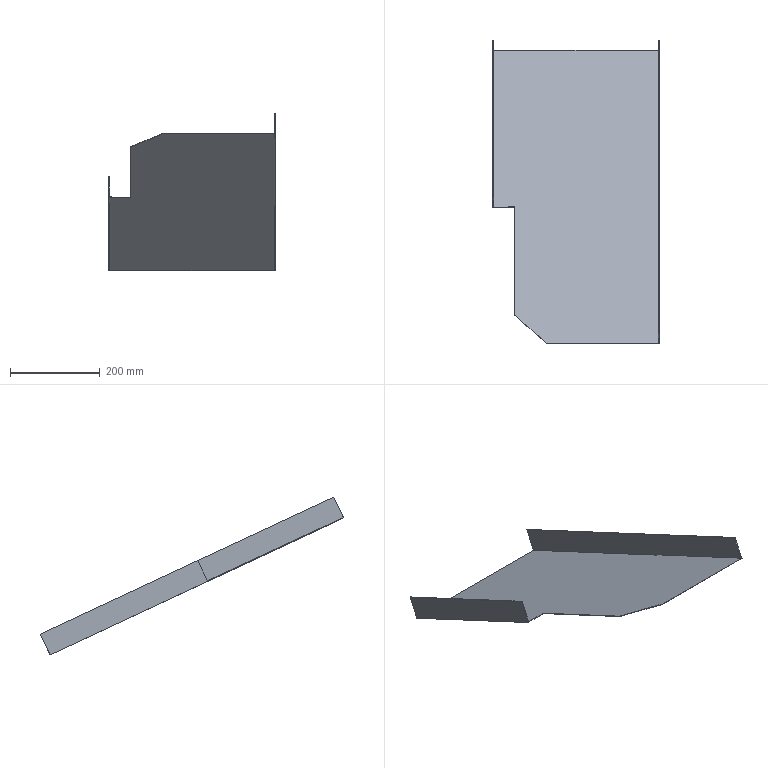Part | NX | features solid 2 | 1 solid | 14 faces | box 370 x 674.707 x 350.792 mm | volume 358626 mm3 | plane 13 | spline 1
STEP:
#1=CARTESIAN_POINT('',(542.,1102.315,-269.141));
#2=VERTEX_POINT('',#1);
#3=CARTESIAN_POINT('',(542.,751.83,-105.707));
#4=VERTEX_POINT('',#3);
#5=CARTESIAN_POINT('',(542.,630.423,-49.094));
#6=DIRECTION('',(0.,0.9063,-0.4226));
#7=VECTOR('',#6,1000.);
#8=LINE('',#5,#7);
#9=EDGE_CURVE('',#2,#4,#8,.F.);
#10=ORIENTED_EDGE('',*,*,#9,.T.);
#11=CARTESIAN_POINT('',(588.755,753.165,-106.33));
#12=VERTEX_POINT('',#11);
#13=CARTESIAN_POINT('',(588.755,753.165,-106.33));
#14=CARTESIAN_POINT('',(586.531,753.112,-106.305));
#15=CARTESIAN_POINT('',(582.277,753.007,-106.256));
#16=CARTESIAN_POINT('',(576.456,752.855,-106.185));
#17=CARTESIAN_POINT('',(572.547,752.747,-106.134));
#18=CARTESIAN_POINT('',(570.076,752.675,-106.101));
#19=CARTESIAN_POINT('',(568.579,752.63,-106.08));
#20=CARTESIAN_POINT('',(565.824,752.548,-106.042));
#21=CARTESIAN_POINT('',(562.091,752.434,-105.989));
#22=CARTESIAN_POINT('',(557.859,752.304,-105.928));
#23=CARTESIAN_POINT('',(554.361,752.195,-105.877));
#24=CARTESIAN_POINT('',(551.213,752.099,-105.832));
#25=CARTESIAN_POINT('',(547.008,751.973,-105.774));
#26=CARTESIAN_POINT('',(543.979,751.886,-105.733));
#27=CARTESIAN_POINT('',(542.,751.83,-105.707));
#28=B_SPLINE_CURVE_WITH_KNOTS('',3,(#13,#14,#15,#16,#17,#18,#19,#20,#21,#22,#23,#24,#25,#26,#27),.UNSPECIFIED.,.F.,.F.,(4,1,1,1,1,1,1,1,1,1,1,1,4),(0.,0.02122,0.04244,0.06367,0.06897,0.07428,0.08489,0.1061,0.1167,0.1273,0.1379,0.1486,0.1698),.UNSPECIFIED.);
#29=EDGE_CURVE('',#12,#4,#28,.T.);
#30=ORIENTED_EDGE('',*,*,#29,.F.);
#31=CARTESIAN_POINT('',(588.755,512.603,5.847));
#32=VERTEX_POINT('',#31);
#33=CARTESIAN_POINT('',(588.755,630.423,-49.094));
#34=DIRECTION('',(0.,-0.9063,0.4226));
#35=VECTOR('',#34,1000.);
#36=LINE('',#33,#35);
#37=EDGE_CURVE('',#32,#12,#36,.F.);
#38=ORIENTED_EDGE('',*,*,#37,.F.);
#39=CARTESIAN_POINT('',(658.755,449.161,35.43));
#40=VERTEX_POINT('',#39);
#41=CARTESIAN_POINT('',(-320.623,1336.778,-378.473));
#42=DIRECTION('',(0.7071,-0.6409,0.2988));
#43=VECTOR('',#42,1000.);
#44=LINE('',#41,#43);
#45=EDGE_CURVE('',#40,#32,#44,.F.);
#46=ORIENTED_EDGE('',*,*,#45,.F.);
#47=CARTESIAN_POINT('',(908.,449.161,35.43));
#48=VERTEX_POINT('',#47);
#49=CARTESIAN_POINT('',(-1100.,449.161,35.43));
#50=DIRECTION('',(1.,0.,0.));
#51=VECTOR('',#50,1000.);
#52=LINE('',#49,#51);
#53=EDGE_CURVE('',#48,#40,#52,.F.);
#54=ORIENTED_EDGE('',*,*,#53,.F.);
#55=CARTESIAN_POINT('',(908.,1102.315,-269.141));
#56=VERTEX_POINT('',#55);
#57=CARTESIAN_POINT('',(908.,630.423,-49.094));
#58=DIRECTION('',(0.,0.9063,-0.4226));
#59=VECTOR('',#58,1000.);
#60=LINE('',#57,#59);
#61=EDGE_CURVE('',#56,#48,#60,.F.);
#62=ORIENTED_EDGE('',*,*,#61,.F.);
#63=CARTESIAN_POINT('',(-1100.,1102.315,-269.141));
#64=DIRECTION('',(1.,0.,0.));
#65=VECTOR('',#64,1000.);
#66=LINE('',#63,#65);
#67=EDGE_CURVE('',#56,#2,#66,.F.);
#68=ORIENTED_EDGE('',*,*,#67,.T.);
#69=EDGE_LOOP('',(#10,#30,#38,#46,#54,#62,#68));
#70=FACE_BOUND('',#69,.T.);
#71=CARTESIAN_POINT('',(-1100.,630.423,-49.094));
#72=DIRECTION('',(0.,-0.4226,-0.9063));
#73=DIRECTION('',(0.,-0.9063,0.4226));
#74=AXIS2_PLACEMENT_3D('',#71,#72,#73);
#75=PLANE('',#74);
#76=ADVANCED_FACE('',(#70),#75,.F.);
#77=ORIENTED_EDGE('',*,*,#37,.T.);
#78=CARTESIAN_POINT('',(588.755,752.743,-107.236));
#79=VERTEX_POINT('',#78);
#80=CARTESIAN_POINT('',(588.755,753.165,-106.33));
#81=CARTESIAN_POINT('',(588.755,753.024,-106.632));
#82=CARTESIAN_POINT('',(588.755,752.883,-106.934));
#83=CARTESIAN_POINT('',(588.755,752.743,-107.236));
#84=B_SPLINE_CURVE_WITH_KNOTS('',3,(#80,#81,#82,#83),.UNSPECIFIED.,.F.,.F.,(4,4),(0.,1.),.UNSPECIFIED.);
#85=EDGE_CURVE('',#79,#12,#84,.F.);
#86=ORIENTED_EDGE('',*,*,#85,.F.);
#87=CARTESIAN_POINT('',(588.755,512.18,4.94));
#88=VERTEX_POINT('',#87);
#89=CARTESIAN_POINT('',(588.755,630.,-50.));
#90=DIRECTION('',(0.,-0.9063,0.4226));
#91=VECTOR('',#90,1000.);
#92=LINE('',#89,#91);
#93=EDGE_CURVE('',#88,#79,#92,.F.);
#94=ORIENTED_EDGE('',*,*,#93,.F.);
#95=CARTESIAN_POINT('',(588.755,512.18,4.94));
#96=DIRECTION('',(0.,-0.4226,-0.9063));
#97=VECTOR('',#96,1000.);
#98=LINE('',#95,#97);
#99=EDGE_CURVE('',#32,#88,#98,.T.);
#100=ORIENTED_EDGE('',*,*,#99,.F.);
#101=EDGE_LOOP('',(#77,#86,#94,#100));
#102=FACE_BOUND('',#101,.T.);
#103=CARTESIAN_POINT('',(588.755,630.,-50.));
#104=DIRECTION('',(-1.,0.,0.));
#105=DIRECTION('',(0.,0.,1.));
#106=AXIS2_PLACEMENT_3D('',#103,#104,#105);
#107=PLANE('',#106);
#108=ADVANCED_FACE('',(#102),#107,.T.);
#109=CARTESIAN_POINT('',(542.,751.407,-106.613));
#110=VERTEX_POINT('',#109);
#111=CARTESIAN_POINT('',(542.,751.407,-106.613));
#112=DIRECTION('',(0.,0.4226,0.9063));
#113=VECTOR('',#112,1000.);
#114=LINE('',#111,#113);
#115=EDGE_CURVE('',#4,#110,#114,.F.);
#116=ORIENTED_EDGE('',*,*,#115,.T.);
#117=CARTESIAN_POINT('',(588.755,752.743,-107.236));
#118=CARTESIAN_POINT('',(586.531,752.689,-107.211));
#119=CARTESIAN_POINT('',(582.277,752.584,-107.162));
#120=CARTESIAN_POINT('',(576.456,752.433,-107.091));
#121=CARTESIAN_POINT('',(572.547,752.324,-107.041));
#122=CARTESIAN_POINT('',(570.076,752.252,-107.007));
#123=CARTESIAN_POINT('',(568.579,752.208,-106.986));
#124=CARTESIAN_POINT('',(565.824,752.125,-106.948));
#125=CARTESIAN_POINT('',(562.091,752.012,-106.895));
#126=CARTESIAN_POINT('',(557.859,751.881,-106.834));
#127=CARTESIAN_POINT('',(554.361,751.773,-106.783));
#128=CARTESIAN_POINT('',(551.213,751.676,-106.739));
#129=CARTESIAN_POINT('',(547.008,751.55,-106.68));
#130=CARTESIAN_POINT('',(543.979,751.463,-106.639));
#131=CARTESIAN_POINT('',(542.,751.407,-106.613));
#132=B_SPLINE_CURVE_WITH_KNOTS('',3,(#117,#118,#119,#120,#121,#122,#123,#124,#125,#126,#127,#128,#129,#130,#131),.UNSPECIFIED.,.F.,.F.,(4,1,1,1,1,1,1,1,1,1,1,1,4),(0.,0.02122,0.04244,0.06367,0.06897,0.07428,0.08489,0.1061,0.1167,0.1273,0.1379,0.1486,0.1698),.UNSPECIFIED.);
#133=EDGE_CURVE('',#79,#110,#132,.T.);
#134=ORIENTED_EDGE('',*,*,#133,.F.);
#135=ORIENTED_EDGE('',*,*,#85,.T.);
#136=ORIENTED_EDGE('',*,*,#29,.T.);
#137=EDGE_LOOP('',(#116,#134,#135,#136));
#138=FACE_BOUND('',#137,.T.);
#139=CARTESIAN_POINT('',(588.755,752.743,-107.236));
#140=CARTESIAN_POINT('',(588.755,753.165,-106.33));
#141=CARTESIAN_POINT('',(586.531,752.689,-107.211));
#142=CARTESIAN_POINT('',(586.531,753.112,-106.305));
#143=CARTESIAN_POINT('',(582.277,752.584,-107.162));
#144=CARTESIAN_POINT('',(582.277,753.007,-106.256));
#145=CARTESIAN_POINT('',(576.456,752.433,-107.091));
#146=CARTESIAN_POINT('',(576.456,752.855,-106.185));
#147=CARTESIAN_POINT('',(572.547,752.324,-107.041));
#148=CARTESIAN_POINT('',(572.547,752.747,-106.134));
#149=CARTESIAN_POINT('',(570.076,752.252,-107.007));
#150=CARTESIAN_POINT('',(570.076,752.675,-106.101));
#151=CARTESIAN_POINT('',(568.579,752.208,-106.986));
#152=CARTESIAN_POINT('',(568.579,752.63,-106.08));
#153=CARTESIAN_POINT('',(565.824,752.125,-106.948));
#154=CARTESIAN_POINT('',(565.824,752.548,-106.042));
#155=CARTESIAN_POINT('',(562.091,752.012,-106.895));
#156=CARTESIAN_POINT('',(562.091,752.434,-105.989));
#157=CARTESIAN_POINT('',(557.859,751.881,-106.834));
#158=CARTESIAN_POINT('',(557.859,752.304,-105.928));
#159=CARTESIAN_POINT('',(554.361,751.773,-106.783));
#160=CARTESIAN_POINT('',(554.361,752.195,-105.877));
#161=CARTESIAN_POINT('',(551.213,751.676,-106.739));
#162=CARTESIAN_POINT('',(551.213,752.099,-105.832));
#163=CARTESIAN_POINT('',(547.008,751.55,-106.68));
#164=CARTESIAN_POINT('',(547.008,751.973,-105.774));
#165=CARTESIAN_POINT('',(543.979,751.463,-106.639));
#166=CARTESIAN_POINT('',(543.979,751.886,-105.733));
#167=CARTESIAN_POINT('',(542.,751.407,-106.613));
#168=CARTESIAN_POINT('',(542.,751.83,-105.707));
#169=B_SPLINE_SURFACE_WITH_KNOTS('',3,1,((#139,#140),(#141,#142),(#143,#144),(#145,#146),(#147,#148),(#149,#150),(#151,#152),(#153,#154),(#155,#156),(#157,#158),(#159,#160),(#161,#162),(#163,#164),(#165,#166),(#167,#168)),.SURF_OF_LINEAR_EXTRUSION.,.F.,.F.,.F.,(4,1,1,1,1,1,1,1,1,1,1,1,4),(2,2),(0.,0.02122,0.04244,0.06367,0.06897,0.07428,0.08489,0.1061,0.1167,0.1273,0.1379,0.1486,0.1698),(0.,1.),.UNSPECIFIED.);
#170=ADVANCED_FACE('',(#138),#169,.F.);
#171=ORIENTED_EDGE('',*,*,#67,.F.);
#172=CARTESIAN_POINT('',(908.,1123.446,-223.825));
#173=VERTEX_POINT('',#172);
#174=CARTESIAN_POINT('',(908.,1123.446,-223.825));
#175=DIRECTION('',(0.,-0.4226,-0.9063));
#176=VECTOR('',#175,1000.);
#177=LINE('',#174,#176);
#178=EDGE_CURVE('',#173,#56,#177,.T.);
#179=ORIENTED_EDGE('',*,*,#178,.F.);
#180=CARTESIAN_POINT('',(910.,1123.446,-223.825));
#181=VERTEX_POINT('',#180);
#182=CARTESIAN_POINT('',(910.,1123.446,-223.825));
#183=DIRECTION('',(1.,0.,0.));
#184=VECTOR('',#183,1000.);
#185=LINE('',#182,#184);
#186=EDGE_CURVE('',#181,#173,#185,.F.);
#187=ORIENTED_EDGE('',*,*,#186,.F.);
#188=CARTESIAN_POINT('',(910.,1101.892,-270.047));
#189=VERTEX_POINT('',#188);
#190=CARTESIAN_POINT('',(910.,1101.892,-270.047));
#191=DIRECTION('',(0.,0.4226,0.9063));
#192=VECTOR('',#191,1000.);
#193=LINE('',#190,#192);
#194=EDGE_CURVE('',#189,#181,#193,.T.);
#195=ORIENTED_EDGE('',*,*,#194,.F.);
#196=CARTESIAN_POINT('',(540.,1101.892,-270.047));
#197=VERTEX_POINT('',#196);
#198=CARTESIAN_POINT('',(-1100.,1101.892,-270.047));
#199=DIRECTION('',(1.,0.,0.));
#200=VECTOR('',#199,1000.);
#201=LINE('',#198,#200);
#202=EDGE_CURVE('',#189,#197,#201,.F.);
#203=ORIENTED_EDGE('',*,*,#202,.T.);
#204=CARTESIAN_POINT('',(540.,1123.446,-223.825));
#205=VERTEX_POINT('',#204);
#206=CARTESIAN_POINT('',(540.,1101.892,-270.047));
#207=DIRECTION('',(0.,-0.4226,-0.9063));
#208=VECTOR('',#207,1000.);
#209=LINE('',#206,#208);
#210=EDGE_CURVE('',#205,#197,#209,.T.);
#211=ORIENTED_EDGE('',*,*,#210,.F.);
#212=CARTESIAN_POINT('',(542.,1123.446,-223.825));
#213=VERTEX_POINT('',#212);
#214=CARTESIAN_POINT('',(540.,1123.446,-223.825));
#215=DIRECTION('',(1.,0.,0.));
#216=VECTOR('',#215,1000.);
#217=LINE('',#214,#216);
#218=EDGE_CURVE('',#213,#205,#217,.F.);
#219=ORIENTED_EDGE('',*,*,#218,.F.);
#220=CARTESIAN_POINT('',(542.,1101.892,-270.047));
#221=DIRECTION('',(0.,0.4226,0.9063));
#222=VECTOR('',#221,1000.);
#223=LINE('',#220,#222);
#224=EDGE_CURVE('',#2,#213,#223,.T.);
#225=ORIENTED_EDGE('',*,*,#224,.F.);
#226=EDGE_LOOP('',(#171,#179,#187,#195,#203,#211,#219,#225));
#227=FACE_BOUND('',#226,.T.);
#228=CARTESIAN_POINT('',(-1100.,1101.892,-270.047));
#229=DIRECTION('',(0.,-0.9063,0.4226));
#230=DIRECTION('',(0.,0.4226,0.9063));
#231=AXIS2_PLACEMENT_3D('',#228,#229,#230);
#232=PLANE('',#231);
#233=ADVANCED_FACE('',(#227),#232,.F.);
#234=CARTESIAN_POINT('',(910.,448.738,34.524));
#235=VERTEX_POINT('',#234);
#236=CARTESIAN_POINT('',(910.,470.292,80.745));
#237=VERTEX_POINT('',#236);
#238=CARTESIAN_POINT('',(910.,448.738,34.524));
#239=DIRECTION('',(0.,0.4226,0.9063));
#240=VECTOR('',#239,1000.);
#241=LINE('',#238,#240);
#242=EDGE_CURVE('',#235,#237,#241,.T.);
#243=ORIENTED_EDGE('',*,*,#242,.F.);
#244=CARTESIAN_POINT('',(910.,630.,-50.));
#245=DIRECTION('',(0.,-0.9063,0.4226));
#246=VECTOR('',#245,1000.);
#247=LINE('',#244,#246);
#248=EDGE_CURVE('',#235,#189,#247,.F.);
#249=ORIENTED_EDGE('',*,*,#248,.T.);
#250=ORIENTED_EDGE('',*,*,#194,.T.);
#251=CARTESIAN_POINT('',(910.,470.292,80.745));
#252=DIRECTION('',(0.,0.9063,-0.4226));
#253=VECTOR('',#252,1000.);
#254=LINE('',#251,#253);
#255=EDGE_CURVE('',#237,#181,#254,.T.);
#256=ORIENTED_EDGE('',*,*,#255,.F.);
#257=EDGE_LOOP('',(#243,#249,#250,#256));
#258=FACE_BOUND('',#257,.T.);
#259=CARTESIAN_POINT('',(910.,630.,-50.));
#260=DIRECTION('',(-1.,0.,0.));
#261=DIRECTION('',(0.,0.,1.));
#262=AXIS2_PLACEMENT_3D('',#259,#260,#261);
#263=PLANE('',#262);
#264=ADVANCED_FACE('',(#258),#263,.F.);
#265=ORIENTED_EDGE('',*,*,#242,.T.);
#266=CARTESIAN_POINT('',(908.,470.292,80.745));
#267=VERTEX_POINT('',#266);
#268=CARTESIAN_POINT('',(910.,470.292,80.745));
#269=DIRECTION('',(1.,0.,0.));
#270=VECTOR('',#269,1000.);
#271=LINE('',#268,#270);
#272=EDGE_CURVE('',#237,#267,#271,.F.);
#273=ORIENTED_EDGE('',*,*,#272,.T.);
#274=CARTESIAN_POINT('',(908.,470.292,80.745));
#275=DIRECTION('',(0.,-0.4226,-0.9063));
#276=VECTOR('',#275,1000.);
#277=LINE('',#274,#276);
#278=EDGE_CURVE('',#267,#48,#277,.T.);
#279=ORIENTED_EDGE('',*,*,#278,.T.);
#280=ORIENTED_EDGE('',*,*,#53,.T.);
#281=CARTESIAN_POINT('',(658.755,448.738,34.524));
#282=VERTEX_POINT('',#281);
#283=CARTESIAN_POINT('',(658.755,448.738,34.524));
#284=DIRECTION('',(0.,0.4226,0.9063));
#285=VECTOR('',#284,1000.);
#286=LINE('',#283,#285);
#287=EDGE_CURVE('',#282,#40,#286,.T.);
#288=ORIENTED_EDGE('',*,*,#287,.F.);
#289=CARTESIAN_POINT('',(-1100.,448.738,34.524));
#290=DIRECTION('',(-1.,0.,0.));
#291=VECTOR('',#290,1000.);
#292=LINE('',#289,#291);
#293=EDGE_CURVE('',#282,#235,#292,.F.);
#294=ORIENTED_EDGE('',*,*,#293,.T.);
#295=EDGE_LOOP('',(#265,#273,#279,#280,#288,#294));
#296=FACE_BOUND('',#295,.T.);
#297=CARTESIAN_POINT('',(-1100.,448.738,34.524));
#298=DIRECTION('',(0.,0.9063,-0.4226));
#299=DIRECTION('',(0.,-0.4226,-0.9063));
#300=AXIS2_PLACEMENT_3D('',#297,#298,#299);
#301=PLANE('',#300);
#302=ADVANCED_FACE('',(#296),#301,.F.);
#303=ORIENTED_EDGE('',*,*,#202,.F.);
#304=ORIENTED_EDGE('',*,*,#248,.F.);
#305=ORIENTED_EDGE('',*,*,#293,.F.);
#306=CARTESIAN_POINT('',(708.755,403.423,55.655));
#307=DIRECTION('',(-0.7071,0.6409,-0.2988));
#308=VECTOR('',#307,1000.);
#309=LINE('',#306,#308);
#310=EDGE_CURVE('',#88,#282,#309,.F.);
#311=ORIENTED_EDGE('',*,*,#310,.F.);
#312=ORIENTED_EDGE('',*,*,#93,.T.);
#313=ORIENTED_EDGE('',*,*,#133,.T.);
#314=CARTESIAN_POINT('',(542.,751.352,-106.587));
#315=VERTEX_POINT('',#314);
#316=CARTESIAN_POINT('',(542.,1101.892,-270.047));
#317=DIRECTION('',(0.,-0.9063,0.4226));
#318=VECTOR('',#317,1000.);
#319=LINE('',#316,#318);
#320=EDGE_CURVE('',#110,#315,#319,.T.);
#321=ORIENTED_EDGE('',*,*,#320,.T.);
#322=CARTESIAN_POINT('',(540.,751.352,-106.587));
#323=VERTEX_POINT('',#322);
#324=CARTESIAN_POINT('',(540.,751.352,-106.587));
#325=DIRECTION('',(1.,0.,0.));
#326=VECTOR('',#325,1000.);
#327=LINE('',#324,#326);
#328=EDGE_CURVE('',#315,#323,#327,.F.);
#329=ORIENTED_EDGE('',*,*,#328,.T.);
#330=CARTESIAN_POINT('',(540.,630.,-50.));
#331=DIRECTION('',(0.,0.9063,-0.4226));
#332=VECTOR('',#331,1000.);
#333=LINE('',#330,#332);
#334=EDGE_CURVE('',#197,#323,#333,.F.);
#335=ORIENTED_EDGE('',*,*,#334,.F.);
#336=EDGE_LOOP('',(#303,#304,#305,#311,#312,#313,#321,#329,#335));
#337=FACE_BOUND('',#336,.T.);
#338=CARTESIAN_POINT('',(-1100.,630.,-50.));
#339=DIRECTION('',(0.,-0.4226,-0.9063));
#340=DIRECTION('',(0.,-0.9063,0.4226));
#341=AXIS2_PLACEMENT_3D('',#338,#339,#340);
#342=PLANE('',#341);
#343=ADVANCED_FACE('',(#337),#342,.T.);
#344=ORIENTED_EDGE('',*,*,#210,.T.);
#345=ORIENTED_EDGE('',*,*,#334,.T.);
#346=CARTESIAN_POINT('',(540.,772.905,-60.365));
#347=VERTEX_POINT('',#346);
#348=CARTESIAN_POINT('',(540.,751.352,-106.587));
#349=DIRECTION('',(0.,0.4226,0.9063));
#350=VECTOR('',#349,1000.);
#351=LINE('',#348,#350);
#352=EDGE_CURVE('',#347,#323,#351,.F.);
#353=ORIENTED_EDGE('',*,*,#352,.F.);
#354=CARTESIAN_POINT('',(540.,1123.446,-223.825));
#355=DIRECTION('',(0.,-0.9063,0.4226));
#356=VECTOR('',#355,1000.);
#357=LINE('',#354,#356);
#358=EDGE_CURVE('',#205,#347,#357,.T.);
#359=ORIENTED_EDGE('',*,*,#358,.F.);
#360=EDGE_LOOP('',(#344,#345,#353,#359));
#361=FACE_BOUND('',#360,.T.);
#362=CARTESIAN_POINT('',(540.,0.,0.));
#363=DIRECTION('',(1.,0.,0.));
#364=DIRECTION('',(0.,0.,-1.));
#365=AXIS2_PLACEMENT_3D('',#362,#363,#364);
#366=PLANE('',#365);
#367=ADVANCED_FACE('',(#361),#366,.F.);
#368=ORIENTED_EDGE('',*,*,#310,.T.);
#369=ORIENTED_EDGE('',*,*,#287,.T.);
#370=ORIENTED_EDGE('',*,*,#45,.T.);
#371=ORIENTED_EDGE('',*,*,#99,.T.);
#372=EDGE_LOOP('',(#368,#369,#370,#371));
#373=FACE_BOUND('',#372,.T.);
#374=CARTESIAN_POINT('',(708.755,403.423,55.655));
#375=DIRECTION('',(-0.7071,-0.6409,0.2988));
#376=DIRECTION('',(-0.6715,0.741,0.));
#377=AXIS2_PLACEMENT_3D('',#374,#375,#376);
#378=PLANE('',#377);
#379=ADVANCED_FACE('',(#373),#378,.T.);
#380=ORIENTED_EDGE('',*,*,#272,.F.);
#381=ORIENTED_EDGE('',*,*,#255,.T.);
#382=ORIENTED_EDGE('',*,*,#186,.T.);
#383=CARTESIAN_POINT('',(908.,470.292,80.745));
#384=DIRECTION('',(0.,0.9063,-0.4226));
#385=VECTOR('',#384,1000.);
#386=LINE('',#383,#385);
#387=EDGE_CURVE('',#267,#173,#386,.T.);
#388=ORIENTED_EDGE('',*,*,#387,.F.);
#389=EDGE_LOOP('',(#380,#381,#382,#388));
#390=FACE_BOUND('',#389,.T.);
#391=CARTESIAN_POINT('',(910.,470.292,80.745));
#392=DIRECTION('',(0.,0.4226,0.9063));
#393=DIRECTION('',(0.,0.9063,-0.4226));
#394=AXIS2_PLACEMENT_3D('',#391,#392,#393);
#395=PLANE('',#394);
#396=ADVANCED_FACE('',(#390),#395,.T.);
#397=ORIENTED_EDGE('',*,*,#61,.T.);
#398=ORIENTED_EDGE('',*,*,#278,.F.);
#399=ORIENTED_EDGE('',*,*,#387,.T.);
#400=ORIENTED_EDGE('',*,*,#178,.T.);
#401=EDGE_LOOP('',(#397,#398,#399,#400));
#402=FACE_BOUND('',#401,.T.);
#403=CARTESIAN_POINT('',(908.,470.292,80.745));
#404=DIRECTION('',(1.,0.,0.));
#405=DIRECTION('',(0.,0.,-1.));
#406=AXIS2_PLACEMENT_3D('',#403,#404,#405);
#407=PLANE('',#406);
#408=ADVANCED_FACE('',(#402),#407,.F.);
#409=ORIENTED_EDGE('',*,*,#328,.F.);
#410=CARTESIAN_POINT('',(542.,772.905,-60.365));
#411=VERTEX_POINT('',#410);
#412=CARTESIAN_POINT('',(542.,751.352,-106.587));
#413=DIRECTION('',(0.,0.4226,0.9063));
#414=VECTOR('',#413,1000.);
#415=LINE('',#412,#414);
#416=EDGE_CURVE('',#315,#411,#415,.T.);
#417=ORIENTED_EDGE('',*,*,#416,.T.);
#418=CARTESIAN_POINT('',(540.,772.905,-60.365));
#419=DIRECTION('',(1.,0.,0.));
#420=VECTOR('',#419,1000.);
#421=LINE('',#418,#420);
#422=EDGE_CURVE('',#411,#347,#421,.F.);
#423=ORIENTED_EDGE('',*,*,#422,.T.);
#424=ORIENTED_EDGE('',*,*,#352,.T.);
#425=EDGE_LOOP('',(#409,#417,#423,#424));
#426=FACE_BOUND('',#425,.T.);
#427=CARTESIAN_POINT('',(540.,751.352,-106.587));
#428=DIRECTION('',(0.,-0.9063,0.4226));
#429=DIRECTION('',(0.,0.4226,0.9063));
#430=AXIS2_PLACEMENT_3D('',#427,#428,#429);
#431=PLANE('',#430);
#432=ADVANCED_FACE('',(#426),#431,.T.);
#433=ORIENTED_EDGE('',*,*,#422,.F.);
#434=CARTESIAN_POINT('',(542.,1123.446,-223.825));
#435=DIRECTION('',(0.,-0.9063,0.4226));
#436=VECTOR('',#435,1000.);
#437=LINE('',#434,#436);
#438=EDGE_CURVE('',#213,#411,#437,.T.);
#439=ORIENTED_EDGE('',*,*,#438,.F.);
#440=ORIENTED_EDGE('',*,*,#218,.T.);
#441=ORIENTED_EDGE('',*,*,#358,.T.);
#442=EDGE_LOOP('',(#433,#439,#440,#441));
#443=FACE_BOUND('',#442,.T.);
#444=CARTESIAN_POINT('',(540.,1123.446,-223.825));
#445=DIRECTION('',(0.,-0.4226,-0.9063));
#446=DIRECTION('',(0.,-0.9063,0.4226));
#447=AXIS2_PLACEMENT_3D('',#444,#445,#446);
#448=PLANE('',#447);
#449=ADVANCED_FACE('',(#443),#448,.F.);
#450=ORIENTED_EDGE('',*,*,#224,.T.);
#451=ORIENTED_EDGE('',*,*,#438,.T.);
#452=ORIENTED_EDGE('',*,*,#416,.F.);
#453=ORIENTED_EDGE('',*,*,#320,.F.);
#454=ORIENTED_EDGE('',*,*,#115,.F.);
#455=ORIENTED_EDGE('',*,*,#9,.F.);
#456=EDGE_LOOP('',(#450,#451,#452,#453,#454,#455));
#457=FACE_BOUND('',#456,.T.);
#458=CARTESIAN_POINT('',(542.,1101.892,-270.047));
#459=DIRECTION('',(1.,0.,0.));
#460=DIRECTION('',(0.,0.,-1.));
#461=AXIS2_PLACEMENT_3D('',#458,#459,#460);
#462=PLANE('',#461);
#463=ADVANCED_FACE('',(#457),#462,.T.);
#464=CLOSED_SHELL('',(#76,#108,#170,#233,#264,#302,#343,#367,#379,#396,#408,#432,#449,#463));
#465=MANIFOLD_SOLID_BREP('',#464);
#466=(LENGTH_UNIT()NAMED_UNIT(*)SI_UNIT(.MILLI.,.METRE.));
#467=UNCERTAINTY_MEASURE_WITH_UNIT(LENGTH_MEASURE(0.0508),#466,'','');
#468=(NAMED_UNIT(*)PLANE_ANGLE_UNIT()SI_UNIT($,.RADIAN.));
#469=(NAMED_UNIT(*)SI_UNIT($,.STERADIAN.)SOLID_ANGLE_UNIT());
#470=(GEOMETRIC_REPRESENTATION_CONTEXT(3)GLOBAL_UNCERTAINTY_ASSIGNED_CONTEXT((#467))GLOBAL_UNIT_ASSIGNED_CONTEXT((#466,#468,#469))REPRESENTATION_CONTEXT('',''));
#471=ADVANCED_BREP_SHAPE_REPRESENTATION('',(#465),#470);